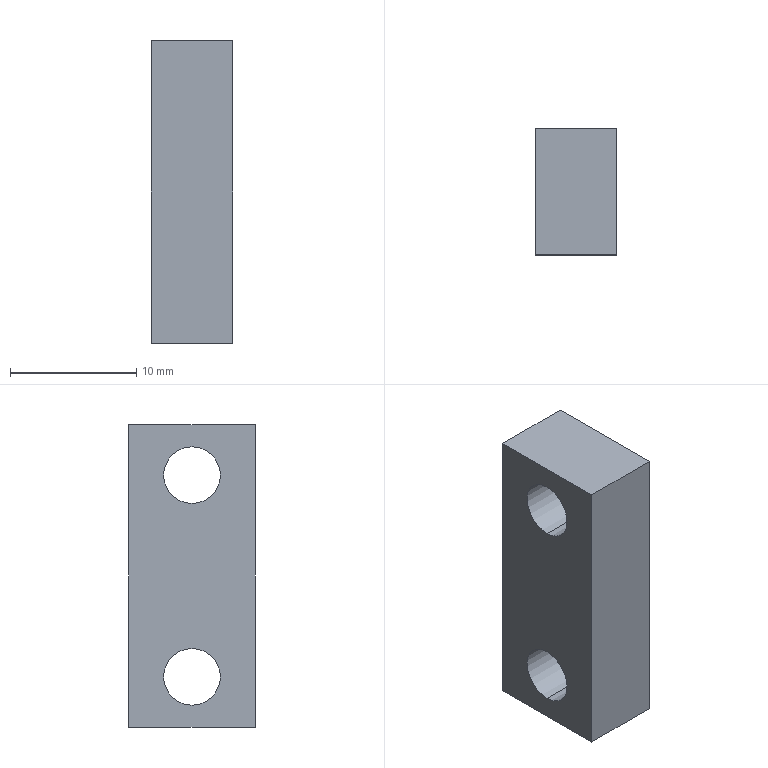Part | STEP file | PN_0044 spacer | 1 solid | 10 faces | box 6.5 x 10 x 24 mm | volume 1353 mm3 | plane 6 | cylinder 4 | commonest cylinder face diameters 4.5 x4
STEP:
#1=CARTESIAN_POINT('',(0.,0.,0.));
#2=DIRECTION('',(0.,0.,1.));
#3=DIRECTION('',(1.,0.,0.));
#4=AXIS2_PLACEMENT_3D('',#1,#2,#3);
#5=CARTESIAN_POINT('',(0.,5.,5.75));
#6=VERTEX_POINT('',#5);
#7=CARTESIAN_POINT('',(6.5,5.,5.75));
#8=VERTEX_POINT('',#7);
#9=CARTESIAN_POINT('',(6.5,5.,5.75));
#10=DIRECTION('',(1.,0.,0.));
#11=VECTOR('',#10,1.);
#12=LINE('',#9,#11);
#13=CARTESIAN_POINT('',(6.5,5.,8.));
#14=DIRECTION('',(1.,0.,0.));
#15=DIRECTION('',(0.,0.,-1.));
#16=AXIS2_PLACEMENT_3D('',#13,#14,#15);
#17=CYLINDRICAL_SURFACE('',#16,2.25);
#18=CARTESIAN_POINT('',(6.283,0.));
#19=DIRECTION('',(0.,1.));
#20=VECTOR('',#19,1.);
#21=LINE('',#18,#20);
#22=(GEOMETRIC_REPRESENTATION_CONTEXT(2)PARAMETRIC_REPRESENTATION_CONTEXT()REPRESENTATION_CONTEXT('',''));
#23=DEFINITIONAL_REPRESENTATION('',(#21),#22);
#24=PCURVE('',#17,#23);
#25=CARTESIAN_POINT('',(6.5,5.,8.));
#26=DIRECTION('',(1.,0.,0.));
#27=DIRECTION('',(0.,0.,-1.));
#28=AXIS2_PLACEMENT_3D('',#25,#26,#27);
#29=CYLINDRICAL_SURFACE('',#28,2.25);
#30=CARTESIAN_POINT('',(0.,0.));
#31=DIRECTION('',(0.,1.));
#32=VECTOR('',#31,1.);
#33=LINE('',#30,#32);
#34=(GEOMETRIC_REPRESENTATION_CONTEXT(2)PARAMETRIC_REPRESENTATION_CONTEXT()REPRESENTATION_CONTEXT('',''));
#35=DEFINITIONAL_REPRESENTATION('',(#33),#34);
#36=PCURVE('',#29,#35);
#37=SURFACE_CURVE('',#12,(#24,#36),.PCURVE_S1.);
#38=EDGE_CURVE('',#6,#8,#37,.T.);
#39=ORIENTED_EDGE('',*,*,#38,.T.);
#40=CARTESIAN_POINT('',(6.5,5.,10.25));
#41=VERTEX_POINT('',#40);
#42=CARTESIAN_POINT('',(6.5,5.,8.));
#43=DIRECTION('',(1.,0.,0.));
#44=DIRECTION('',(0.,0.,-1.));
#45=AXIS2_PLACEMENT_3D('',#42,#43,#44);
#46=CIRCLE('',#45,2.25);
#47=CARTESIAN_POINT('',(0.,0.));
#48=DIRECTION('',(1.,0.));
#49=VECTOR('',#48,1.);
#50=LINE('',#47,#49);
#51=(GEOMETRIC_REPRESENTATION_CONTEXT(2)PARAMETRIC_REPRESENTATION_CONTEXT()REPRESENTATION_CONTEXT('',''));
#52=DEFINITIONAL_REPRESENTATION('',(#50),#51);
#53=PCURVE('',#17,#52);
#54=CARTESIAN_POINT('',(6.5,0.,0.));
#55=DIRECTION('',(-1.,0.,0.));
#56=DIRECTION('',(0.,0.,1.));
#57=AXIS2_PLACEMENT_3D('',#54,#55,#56);
#58=PLANE('',#57);
#59=CARTESIAN_POINT('',(5.75,5.));
#60=CARTESIAN_POINT('',(5.75,8.897));
#61=CARTESIAN_POINT('',(9.125,6.949));
#62=CARTESIAN_POINT('',(12.5,5.));
#63=CARTESIAN_POINT('',(9.125,3.051));
#64=CARTESIAN_POINT('',(5.75,1.103));
#65=CARTESIAN_POINT('',(5.75,5.));
#66=(BOUNDED_CURVE()B_SPLINE_CURVE(2,(#59,#60,#61,#62,#63,#64,#65),.UNSPECIFIED.,.T.,.F.)B_SPLINE_CURVE_WITH_KNOTS((1,2,2,2,2,1),(-2.094,0.,2.094,4.189,6.283,8.378),.UNSPECIFIED.)CURVE()GEOMETRIC_REPRESENTATION_ITEM()RATIONAL_B_SPLINE_CURVE((1.,0.5,1.,0.5,1.,0.5,1.))REPRESENTATION_ITEM(''));
#67=(GEOMETRIC_REPRESENTATION_CONTEXT(2)PARAMETRIC_REPRESENTATION_CONTEXT()REPRESENTATION_CONTEXT('',''));
#68=DEFINITIONAL_REPRESENTATION('',(#66),#67);
#69=PCURVE('',#58,#68);
#70=SURFACE_CURVE('',#46,(#53,#69),.PCURVE_S1.);
#71=EDGE_CURVE('',#41,#8,#70,.T.);
#72=ORIENTED_EDGE('',*,*,#71,.F.);
#73=CARTESIAN_POINT('',(0.,5.,10.25));
#74=VERTEX_POINT('',#73);
#75=CARTESIAN_POINT('',(6.5,5.,10.25));
#76=DIRECTION('',(1.,0.,0.));
#77=VECTOR('',#76,1.);
#78=LINE('',#75,#77);
#79=CARTESIAN_POINT('',(3.142,0.));
#80=DIRECTION('',(0.,1.));
#81=VECTOR('',#80,1.);
#82=LINE('',#79,#81);
#83=(GEOMETRIC_REPRESENTATION_CONTEXT(2)PARAMETRIC_REPRESENTATION_CONTEXT()REPRESENTATION_CONTEXT('',''));
#84=DEFINITIONAL_REPRESENTATION('',(#82),#83);
#85=PCURVE('',#17,#84);
#86=CARTESIAN_POINT('',(3.142,0.));
#87=DIRECTION('',(0.,1.));
#88=VECTOR('',#87,1.);
#89=LINE('',#86,#88);
#90=(GEOMETRIC_REPRESENTATION_CONTEXT(2)PARAMETRIC_REPRESENTATION_CONTEXT()REPRESENTATION_CONTEXT('',''));
#91=DEFINITIONAL_REPRESENTATION('',(#89),#90);
#92=PCURVE('',#29,#91);
#93=SURFACE_CURVE('',#78,(#85,#92),.PCURVE_S1.);
#94=EDGE_CURVE('',#74,#41,#93,.T.);
#95=ORIENTED_EDGE('',*,*,#94,.F.);
#96=CARTESIAN_POINT('',(0.,5.,8.));
#97=DIRECTION('',(1.,0.,0.));
#98=DIRECTION('',(0.,0.,-1.));
#99=AXIS2_PLACEMENT_3D('',#96,#97,#98);
#100=CIRCLE('',#99,2.25);
#101=CARTESIAN_POINT('',(0.,-6.5));
#102=DIRECTION('',(1.,0.));
#103=VECTOR('',#102,1.);
#104=LINE('',#101,#103);
#105=(GEOMETRIC_REPRESENTATION_CONTEXT(2)PARAMETRIC_REPRESENTATION_CONTEXT()REPRESENTATION_CONTEXT('',''));
#106=DEFINITIONAL_REPRESENTATION('',(#104),#105);
#107=PCURVE('',#17,#106);
#108=CARTESIAN_POINT('',(0.,0.,0.));
#109=DIRECTION('',(-1.,0.,0.));
#110=DIRECTION('',(0.,0.,1.));
#111=AXIS2_PLACEMENT_3D('',#108,#109,#110);
#112=PLANE('',#111);
#113=CARTESIAN_POINT('',(5.75,5.));
#114=CARTESIAN_POINT('',(5.75,8.897));
#115=CARTESIAN_POINT('',(9.125,6.949));
#116=CARTESIAN_POINT('',(12.5,5.));
#117=CARTESIAN_POINT('',(9.125,3.051));
#118=CARTESIAN_POINT('',(5.75,1.103));
#119=CARTESIAN_POINT('',(5.75,5.));
#120=(BOUNDED_CURVE()B_SPLINE_CURVE(2,(#113,#114,#115,#116,#117,#118,#119),.UNSPECIFIED.,.T.,.F.)B_SPLINE_CURVE_WITH_KNOTS((1,2,2,2,2,1),(-2.094,0.,2.094,4.189,6.283,8.378),.UNSPECIFIED.)CURVE()GEOMETRIC_REPRESENTATION_ITEM()RATIONAL_B_SPLINE_CURVE((1.,0.5,1.,0.5,1.,0.5,1.))REPRESENTATION_ITEM(''));
#121=(GEOMETRIC_REPRESENTATION_CONTEXT(2)PARAMETRIC_REPRESENTATION_CONTEXT()REPRESENTATION_CONTEXT('',''));
#122=DEFINITIONAL_REPRESENTATION('',(#120),#121);
#123=PCURVE('',#112,#122);
#124=SURFACE_CURVE('',#100,(#107,#123),.PCURVE_S1.);
#125=EDGE_CURVE('',#74,#6,#124,.T.);
#126=ORIENTED_EDGE('',*,*,#125,.T.);
#127=EDGE_LOOP('',(#39,#72,#95,#126));
#128=FACE_BOUND('',#127,.F.);
#129=ADVANCED_FACE('',(#128),#17,.F.);
#130=CARTESIAN_POINT('',(0.,5.,-10.25));
#131=VERTEX_POINT('',#130);
#132=CARTESIAN_POINT('',(6.5,5.,-10.25));
#133=VERTEX_POINT('',#132);
#134=CARTESIAN_POINT('',(6.5,5.,-10.25));
#135=DIRECTION('',(1.,0.,0.));
#136=VECTOR('',#135,1.);
#137=LINE('',#134,#136);
#138=CARTESIAN_POINT('',(6.5,5.,-8.));
#139=DIRECTION('',(1.,0.,0.));
#140=DIRECTION('',(0.,0.,-1.));
#141=AXIS2_PLACEMENT_3D('',#138,#139,#140);
#142=CYLINDRICAL_SURFACE('',#141,2.25);
#143=CARTESIAN_POINT('',(6.283,0.));
#144=DIRECTION('',(0.,1.));
#145=VECTOR('',#144,1.);
#146=LINE('',#143,#145);
#147=(GEOMETRIC_REPRESENTATION_CONTEXT(2)PARAMETRIC_REPRESENTATION_CONTEXT()REPRESENTATION_CONTEXT('',''));
#148=DEFINITIONAL_REPRESENTATION('',(#146),#147);
#149=PCURVE('',#142,#148);
#150=CARTESIAN_POINT('',(6.5,5.,-8.));
#151=DIRECTION('',(1.,0.,0.));
#152=DIRECTION('',(0.,0.,-1.));
#153=AXIS2_PLACEMENT_3D('',#150,#151,#152);
#154=CYLINDRICAL_SURFACE('',#153,2.25);
#155=CARTESIAN_POINT('',(0.,0.));
#156=DIRECTION('',(0.,1.));
#157=VECTOR('',#156,1.);
#158=LINE('',#155,#157);
#159=(GEOMETRIC_REPRESENTATION_CONTEXT(2)PARAMETRIC_REPRESENTATION_CONTEXT()REPRESENTATION_CONTEXT('',''));
#160=DEFINITIONAL_REPRESENTATION('',(#158),#159);
#161=PCURVE('',#154,#160);
#162=SURFACE_CURVE('',#137,(#149,#161),.PCURVE_S1.);
#163=EDGE_CURVE('',#131,#133,#162,.T.);
#164=ORIENTED_EDGE('',*,*,#163,.T.);
#165=CARTESIAN_POINT('',(6.5,5.,-5.75));
#166=VERTEX_POINT('',#165);
#167=CARTESIAN_POINT('',(6.5,5.,-8.));
#168=DIRECTION('',(1.,0.,0.));
#169=DIRECTION('',(0.,0.,-1.));
#170=AXIS2_PLACEMENT_3D('',#167,#168,#169);
#171=CIRCLE('',#170,2.25);
#172=CARTESIAN_POINT('',(0.,0.));
#173=DIRECTION('',(1.,0.));
#174=VECTOR('',#173,1.);
#175=LINE('',#172,#174);
#176=(GEOMETRIC_REPRESENTATION_CONTEXT(2)PARAMETRIC_REPRESENTATION_CONTEXT()REPRESENTATION_CONTEXT('',''));
#177=DEFINITIONAL_REPRESENTATION('',(#175),#176);
#178=PCURVE('',#142,#177);
#179=CARTESIAN_POINT('',(-10.25,5.));
#180=CARTESIAN_POINT('',(-10.25,8.897));
#181=CARTESIAN_POINT('',(-6.875,6.949));
#182=CARTESIAN_POINT('',(-3.5,5.));
#183=CARTESIAN_POINT('',(-6.875,3.051));
#184=CARTESIAN_POINT('',(-10.25,1.103));
#185=CARTESIAN_POINT('',(-10.25,5.));
#186=(BOUNDED_CURVE()B_SPLINE_CURVE(2,(#179,#180,#181,#182,#183,#184,#185),.UNSPECIFIED.,.T.,.F.)B_SPLINE_CURVE_WITH_KNOTS((1,2,2,2,2,1),(-2.094,0.,2.094,4.189,6.283,8.378),.UNSPECIFIED.)CURVE()GEOMETRIC_REPRESENTATION_ITEM()RATIONAL_B_SPLINE_CURVE((1.,0.5,1.,0.5,1.,0.5,1.))REPRESENTATION_ITEM(''));
#187=(GEOMETRIC_REPRESENTATION_CONTEXT(2)PARAMETRIC_REPRESENTATION_CONTEXT()REPRESENTATION_CONTEXT('',''));
#188=DEFINITIONAL_REPRESENTATION('',(#186),#187);
#189=PCURVE('',#58,#188);
#190=SURFACE_CURVE('',#171,(#178,#189),.PCURVE_S1.);
#191=EDGE_CURVE('',#166,#133,#190,.T.);
#192=ORIENTED_EDGE('',*,*,#191,.F.);
#193=CARTESIAN_POINT('',(0.,5.,-5.75));
#194=VERTEX_POINT('',#193);
#195=CARTESIAN_POINT('',(6.5,5.,-5.75));
#196=DIRECTION('',(1.,0.,0.));
#197=VECTOR('',#196,1.);
#198=LINE('',#195,#197);
#199=CARTESIAN_POINT('',(3.142,0.));
#200=DIRECTION('',(0.,1.));
#201=VECTOR('',#200,1.);
#202=LINE('',#199,#201);
#203=(GEOMETRIC_REPRESENTATION_CONTEXT(2)PARAMETRIC_REPRESENTATION_CONTEXT()REPRESENTATION_CONTEXT('',''));
#204=DEFINITIONAL_REPRESENTATION('',(#202),#203);
#205=PCURVE('',#142,#204);
#206=CARTESIAN_POINT('',(3.142,0.));
#207=DIRECTION('',(0.,1.));
#208=VECTOR('',#207,1.);
#209=LINE('',#206,#208);
#210=(GEOMETRIC_REPRESENTATION_CONTEXT(2)PARAMETRIC_REPRESENTATION_CONTEXT()REPRESENTATION_CONTEXT('',''));
#211=DEFINITIONAL_REPRESENTATION('',(#209),#210);
#212=PCURVE('',#154,#211);
#213=SURFACE_CURVE('',#198,(#205,#212),.PCURVE_S1.);
#214=EDGE_CURVE('',#194,#166,#213,.T.);
#215=ORIENTED_EDGE('',*,*,#214,.F.);
#216=CARTESIAN_POINT('',(0.,5.,-8.));
#217=DIRECTION('',(1.,0.,0.));
#218=DIRECTION('',(0.,0.,-1.));
#219=AXIS2_PLACEMENT_3D('',#216,#217,#218);
#220=CIRCLE('',#219,2.25);
#221=CARTESIAN_POINT('',(0.,-6.5));
#222=DIRECTION('',(1.,0.));
#223=VECTOR('',#222,1.);
#224=LINE('',#221,#223);
#225=(GEOMETRIC_REPRESENTATION_CONTEXT(2)PARAMETRIC_REPRESENTATION_CONTEXT()REPRESENTATION_CONTEXT('',''));
#226=DEFINITIONAL_REPRESENTATION('',(#224),#225);
#227=PCURVE('',#142,#226);
#228=CARTESIAN_POINT('',(-10.25,5.));
#229=CARTESIAN_POINT('',(-10.25,8.897));
#230=CARTESIAN_POINT('',(-6.875,6.949));
#231=CARTESIAN_POINT('',(-3.5,5.));
#232=CARTESIAN_POINT('',(-6.875,3.051));
#233=CARTESIAN_POINT('',(-10.25,1.103));
#234=CARTESIAN_POINT('',(-10.25,5.));
#235=(BOUNDED_CURVE()B_SPLINE_CURVE(2,(#228,#229,#230,#231,#232,#233,#234),.UNSPECIFIED.,.T.,.F.)B_SPLINE_CURVE_WITH_KNOTS((1,2,2,2,2,1),(-2.094,0.,2.094,4.189,6.283,8.378),.UNSPECIFIED.)CURVE()GEOMETRIC_REPRESENTATION_ITEM()RATIONAL_B_SPLINE_CURVE((1.,0.5,1.,0.5,1.,0.5,1.))REPRESENTATION_ITEM(''));
#236=(GEOMETRIC_REPRESENTATION_CONTEXT(2)PARAMETRIC_REPRESENTATION_CONTEXT()REPRESENTATION_CONTEXT('',''));
#237=DEFINITIONAL_REPRESENTATION('',(#235),#236);
#238=PCURVE('',#112,#237);
#239=SURFACE_CURVE('',#220,(#227,#238),.PCURVE_S1.);
#240=EDGE_CURVE('',#194,#131,#239,.T.);
#241=ORIENTED_EDGE('',*,*,#240,.T.);
#242=EDGE_LOOP('',(#164,#192,#215,#241));
#243=FACE_BOUND('',#242,.F.);
#244=ADVANCED_FACE('',(#243),#142,.F.);
#245=CARTESIAN_POINT('',(0.,10.,12.));
#246=VERTEX_POINT('',#245);
#247=CARTESIAN_POINT('',(0.,0.,12.));
#248=VERTEX_POINT('',#247);
#249=CARTESIAN_POINT('',(0.,0.,12.));
#250=DIRECTION('',(0.,-1.,0.));
#251=VECTOR('',#250,1.);
#252=LINE('',#249,#251);
#253=CARTESIAN_POINT('',(6.5,0.,12.));
#254=DIRECTION('',(0.,0.,-1.));
#255=DIRECTION('',(-1.,0.,0.));
#256=AXIS2_PLACEMENT_3D('',#253,#254,#255);
#257=PLANE('',#256);
#258=CARTESIAN_POINT('',(6.5,0.));
#259=DIRECTION('',(0.,-1.));
#260=VECTOR('',#259,1.);
#261=LINE('',#258,#260);
#262=(GEOMETRIC_REPRESENTATION_CONTEXT(2)PARAMETRIC_REPRESENTATION_CONTEXT()REPRESENTATION_CONTEXT('',''));
#263=DEFINITIONAL_REPRESENTATION('',(#261),#262);
#264=PCURVE('',#257,#263);
#265=CARTESIAN_POINT('',(12.,0.));
#266=DIRECTION('',(0.,-1.));
#267=VECTOR('',#266,1.);
#268=LINE('',#265,#267);
#269=(GEOMETRIC_REPRESENTATION_CONTEXT(2)PARAMETRIC_REPRESENTATION_CONTEXT()REPRESENTATION_CONTEXT('',''));
#270=DEFINITIONAL_REPRESENTATION('',(#268),#269);
#271=PCURVE('',#112,#270);
#272=SURFACE_CURVE('',#252,(#264,#271),.PCURVE_S1.);
#273=EDGE_CURVE('',#246,#248,#272,.T.);
#274=ORIENTED_EDGE('',*,*,#273,.T.);
#275=CARTESIAN_POINT('',(6.5,0.,12.));
#276=VERTEX_POINT('',#275);
#277=CARTESIAN_POINT('',(6.5,0.,12.));
#278=DIRECTION('',(-1.,0.,0.));
#279=VECTOR('',#278,1.);
#280=LINE('',#277,#279);
#281=CARTESIAN_POINT('',(0.,0.));
#282=DIRECTION('',(1.,0.));
#283=VECTOR('',#282,1.);
#284=LINE('',#281,#283);
#285=(GEOMETRIC_REPRESENTATION_CONTEXT(2)PARAMETRIC_REPRESENTATION_CONTEXT()REPRESENTATION_CONTEXT('',''));
#286=DEFINITIONAL_REPRESENTATION('',(#284),#285);
#287=PCURVE('',#257,#286);
#288=CARTESIAN_POINT('',(6.5,0.,12.));
#289=DIRECTION('',(0.,1.,0.));
#290=DIRECTION('',(0.,0.,1.));
#291=AXIS2_PLACEMENT_3D('',#288,#289,#290);
#292=PLANE('',#291);
#293=CARTESIAN_POINT('',(0.,0.));
#294=DIRECTION('',(0.,-1.));
#295=VECTOR('',#294,1.);
#296=LINE('',#293,#295);
#297=(GEOMETRIC_REPRESENTATION_CONTEXT(2)PARAMETRIC_REPRESENTATION_CONTEXT()REPRESENTATION_CONTEXT('',''));
#298=DEFINITIONAL_REPRESENTATION('',(#296),#297);
#299=PCURVE('',#292,#298);
#300=SURFACE_CURVE('',#280,(#287,#299),.PCURVE_S1.);
#301=EDGE_CURVE('',#276,#248,#300,.T.);
#302=ORIENTED_EDGE('',*,*,#301,.F.);
#303=CARTESIAN_POINT('',(6.5,10.,12.));
#304=VERTEX_POINT('',#303);
#305=CARTESIAN_POINT('',(6.5,0.,12.));
#306=DIRECTION('',(0.,-1.,0.));
#307=VECTOR('',#306,1.);
#308=LINE('',#305,#307);
#309=CARTESIAN_POINT('',(0.,0.));
#310=DIRECTION('',(0.,-1.));
#311=VECTOR('',#310,1.);
#312=LINE('',#309,#311);
#313=(GEOMETRIC_REPRESENTATION_CONTEXT(2)PARAMETRIC_REPRESENTATION_CONTEXT()REPRESENTATION_CONTEXT('',''));
#314=DEFINITIONAL_REPRESENTATION('',(#312),#313);
#315=PCURVE('',#257,#314);
#316=CARTESIAN_POINT('',(12.,0.));
#317=DIRECTION('',(0.,-1.));
#318=VECTOR('',#317,1.);
#319=LINE('',#316,#318);
#320=(GEOMETRIC_REPRESENTATION_CONTEXT(2)PARAMETRIC_REPRESENTATION_CONTEXT()REPRESENTATION_CONTEXT('',''));
#321=DEFINITIONAL_REPRESENTATION('',(#319),#320);
#322=PCURVE('',#58,#321);
#323=SURFACE_CURVE('',#308,(#315,#322),.PCURVE_S1.);
#324=EDGE_CURVE('',#304,#276,#323,.T.);
#325=ORIENTED_EDGE('',*,*,#324,.F.);
#326=CARTESIAN_POINT('',(6.5,10.,12.));
#327=DIRECTION('',(-1.,0.,0.));
#328=VECTOR('',#327,1.);
#329=LINE('',#326,#328);
#330=CARTESIAN_POINT('',(0.,10.));
#331=DIRECTION('',(1.,0.));
#332=VECTOR('',#331,1.);
#333=LINE('',#330,#332);
#334=(GEOMETRIC_REPRESENTATION_CONTEXT(2)PARAMETRIC_REPRESENTATION_CONTEXT()REPRESENTATION_CONTEXT('',''));
#335=DEFINITIONAL_REPRESENTATION('',(#333),#334);
#336=PCURVE('',#257,#335);
#337=CARTESIAN_POINT('',(6.5,10.,12.));
#338=DIRECTION('',(0.,-1.,0.));
#339=DIRECTION('',(0.,0.,-1.));
#340=AXIS2_PLACEMENT_3D('',#337,#338,#339);
#341=PLANE('',#340);
#342=CARTESIAN_POINT('',(0.,0.));
#343=DIRECTION('',(0.,-1.));
#344=VECTOR('',#343,1.);
#345=LINE('',#342,#344);
#346=(GEOMETRIC_REPRESENTATION_CONTEXT(2)PARAMETRIC_REPRESENTATION_CONTEXT()REPRESENTATION_CONTEXT('',''));
#347=DEFINITIONAL_REPRESENTATION('',(#345),#346);
#348=PCURVE('',#341,#347);
#349=SURFACE_CURVE('',#329,(#336,#348),.PCURVE_S1.);
#350=EDGE_CURVE('',#304,#246,#349,.T.);
#351=ORIENTED_EDGE('',*,*,#350,.T.);
#352=EDGE_LOOP('',(#274,#302,#325,#351));
#353=FACE_BOUND('',#352,.T.);
#354=ADVANCED_FACE('',(#353),#257,.F.);
#355=CARTESIAN_POINT('',(0.,0.,-12.));
#356=VERTEX_POINT('',#355);
#357=CARTESIAN_POINT('',(0.,0.,12.));
#358=DIRECTION('',(0.,0.,-1.));
#359=VECTOR('',#358,1.);
#360=LINE('',#357,#359);
#361=CARTESIAN_POINT('',(0.,-6.5));
#362=DIRECTION('',(-1.,0.));
#363=VECTOR('',#362,1.);
#364=LINE('',#361,#363);
#365=(GEOMETRIC_REPRESENTATION_CONTEXT(2)PARAMETRIC_REPRESENTATION_CONTEXT()REPRESENTATION_CONTEXT('',''));
#366=DEFINITIONAL_REPRESENTATION('',(#364),#365);
#367=PCURVE('',#292,#366);
#368=CARTESIAN_POINT('',(12.,0.));
#369=DIRECTION('',(-1.,0.));
#370=VECTOR('',#369,1.);
#371=LINE('',#368,#370);
#372=(GEOMETRIC_REPRESENTATION_CONTEXT(2)PARAMETRIC_REPRESENTATION_CONTEXT()REPRESENTATION_CONTEXT('',''));
#373=DEFINITIONAL_REPRESENTATION('',(#371),#372);
#374=PCURVE('',#112,#373);
#375=SURFACE_CURVE('',#360,(#367,#374),.PCURVE_S1.);
#376=EDGE_CURVE('',#248,#356,#375,.T.);
#377=ORIENTED_EDGE('',*,*,#376,.T.);
#378=CARTESIAN_POINT('',(6.5,0.,-12.));
#379=VERTEX_POINT('',#378);
#380=CARTESIAN_POINT('',(6.5,0.,-12.));
#381=DIRECTION('',(-1.,0.,0.));
#382=VECTOR('',#381,1.);
#383=LINE('',#380,#382);
#384=CARTESIAN_POINT('',(-24.,0.));
#385=DIRECTION('',(0.,-1.));
#386=VECTOR('',#385,1.);
#387=LINE('',#384,#386);
#388=(GEOMETRIC_REPRESENTATION_CONTEXT(2)PARAMETRIC_REPRESENTATION_CONTEXT()REPRESENTATION_CONTEXT('',''));
#389=DEFINITIONAL_REPRESENTATION('',(#387),#388);
#390=PCURVE('',#292,#389);
#391=CARTESIAN_POINT('',(6.5,0.,-12.));
#392=DIRECTION('',(0.,0.,1.));
#393=DIRECTION('',(1.,0.,0.));
#394=AXIS2_PLACEMENT_3D('',#391,#392,#393);
#395=PLANE('',#394);
#396=CARTESIAN_POINT('',(0.,0.));
#397=DIRECTION('',(-1.,0.));
#398=VECTOR('',#397,1.);
#399=LINE('',#396,#398);
#400=(GEOMETRIC_REPRESENTATION_CONTEXT(2)PARAMETRIC_REPRESENTATION_CONTEXT()REPRESENTATION_CONTEXT('',''));
#401=DEFINITIONAL_REPRESENTATION('',(#399),#400);
#402=PCURVE('',#395,#401);
#403=SURFACE_CURVE('',#383,(#390,#402),.PCURVE_S1.);
#404=EDGE_CURVE('',#379,#356,#403,.T.);
#405=ORIENTED_EDGE('',*,*,#404,.F.);
#406=CARTESIAN_POINT('',(6.5,0.,12.));
#407=DIRECTION('',(0.,0.,-1.));
#408=VECTOR('',#407,1.);
#409=LINE('',#406,#408);
#410=CARTESIAN_POINT('',(0.,0.));
#411=DIRECTION('',(-1.,0.));
#412=VECTOR('',#411,1.);
#413=LINE('',#410,#412);
#414=(GEOMETRIC_REPRESENTATION_CONTEXT(2)PARAMETRIC_REPRESENTATION_CONTEXT()REPRESENTATION_CONTEXT('',''));
#415=DEFINITIONAL_REPRESENTATION('',(#413),#414);
#416=PCURVE('',#292,#415);
#417=CARTESIAN_POINT('',(12.,0.));
#418=DIRECTION('',(-1.,0.));
#419=VECTOR('',#418,1.);
#420=LINE('',#417,#419);
#421=(GEOMETRIC_REPRESENTATION_CONTEXT(2)PARAMETRIC_REPRESENTATION_CONTEXT()REPRESENTATION_CONTEXT('',''));
#422=DEFINITIONAL_REPRESENTATION('',(#420),#421);
#423=PCURVE('',#58,#422);
#424=SURFACE_CURVE('',#409,(#416,#423),.PCURVE_S1.);
#425=EDGE_CURVE('',#276,#379,#424,.T.);
#426=ORIENTED_EDGE('',*,*,#425,.F.);
#427=ORIENTED_EDGE('',*,*,#301,.T.);
#428=EDGE_LOOP('',(#377,#405,#426,#427));
#429=FACE_BOUND('',#428,.T.);
#430=ADVANCED_FACE('',(#429),#292,.F.);
#431=CARTESIAN_POINT('',(0.,10.,-12.));
#432=VERTEX_POINT('',#431);
#433=CARTESIAN_POINT('',(0.,0.,-12.));
#434=DIRECTION('',(0.,1.,0.));
#435=VECTOR('',#434,1.);
#436=LINE('',#433,#435);
#437=CARTESIAN_POINT('',(-6.5,0.));
#438=DIRECTION('',(0.,1.));
#439=VECTOR('',#438,1.);
#440=LINE('',#437,#439);
#441=(GEOMETRIC_REPRESENTATION_CONTEXT(2)PARAMETRIC_REPRESENTATION_CONTEXT()REPRESENTATION_CONTEXT('',''));
#442=DEFINITIONAL_REPRESENTATION('',(#440),#441);
#443=PCURVE('',#395,#442);
#444=CARTESIAN_POINT('',(-12.,0.));
#445=DIRECTION('',(0.,1.));
#446=VECTOR('',#445,1.);
#447=LINE('',#444,#446);
#448=(GEOMETRIC_REPRESENTATION_CONTEXT(2)PARAMETRIC_REPRESENTATION_CONTEXT()REPRESENTATION_CONTEXT('',''));
#449=DEFINITIONAL_REPRESENTATION('',(#447),#448);
#450=PCURVE('',#112,#449);
#451=SURFACE_CURVE('',#436,(#443,#450),.PCURVE_S1.);
#452=EDGE_CURVE('',#356,#432,#451,.T.);
#453=ORIENTED_EDGE('',*,*,#452,.T.);
#454=CARTESIAN_POINT('',(6.5,10.,-12.));
#455=VERTEX_POINT('',#454);
#456=CARTESIAN_POINT('',(6.5,10.,-12.));
#457=DIRECTION('',(-1.,0.,0.));
#458=VECTOR('',#457,1.);
#459=LINE('',#456,#458);
#460=CARTESIAN_POINT('',(0.,10.));
#461=DIRECTION('',(-1.,0.));
#462=VECTOR('',#461,1.);
#463=LINE('',#460,#462);
#464=(GEOMETRIC_REPRESENTATION_CONTEXT(2)PARAMETRIC_REPRESENTATION_CONTEXT()REPRESENTATION_CONTEXT('',''));
#465=DEFINITIONAL_REPRESENTATION('',(#463),#464);
#466=PCURVE('',#395,#465);
#467=CARTESIAN_POINT('',(24.,0.));
#468=DIRECTION('',(0.,-1.));
#469=VECTOR('',#468,1.);
#470=LINE('',#467,#469);
#471=(GEOMETRIC_REPRESENTATION_CONTEXT(2)PARAMETRIC_REPRESENTATION_CONTEXT()REPRESENTATION_CONTEXT('',''));
#472=DEFINITIONAL_REPRESENTATION('',(#470),#471);
#473=PCURVE('',#341,#472);
#474=SURFACE_CURVE('',#459,(#466,#473),.PCURVE_S1.);
#475=EDGE_CURVE('',#455,#432,#474,.T.);
#476=ORIENTED_EDGE('',*,*,#475,.F.);
#477=CARTESIAN_POINT('',(6.5,0.,-12.));
#478=DIRECTION('',(0.,1.,0.));
#479=VECTOR('',#478,1.);
#480=LINE('',#477,#479);
#481=CARTESIAN_POINT('',(0.,0.));
#482=DIRECTION('',(0.,1.));
#483=VECTOR('',#482,1.);
#484=LINE('',#481,#483);
#485=(GEOMETRIC_REPRESENTATION_CONTEXT(2)PARAMETRIC_REPRESENTATION_CONTEXT()REPRESENTATION_CONTEXT('',''));
#486=DEFINITIONAL_REPRESENTATION('',(#484),#485);
#487=PCURVE('',#395,#486);
#488=CARTESIAN_POINT('',(-12.,0.));
#489=DIRECTION('',(0.,1.));
#490=VECTOR('',#489,1.);
#491=LINE('',#488,#490);
#492=(GEOMETRIC_REPRESENTATION_CONTEXT(2)PARAMETRIC_REPRESENTATION_CONTEXT()REPRESENTATION_CONTEXT('',''));
#493=DEFINITIONAL_REPRESENTATION('',(#491),#492);
#494=PCURVE('',#58,#493);
#495=SURFACE_CURVE('',#480,(#487,#494),.PCURVE_S1.);
#496=EDGE_CURVE('',#379,#455,#495,.T.);
#497=ORIENTED_EDGE('',*,*,#496,.F.);
#498=ORIENTED_EDGE('',*,*,#404,.T.);
#499=EDGE_LOOP('',(#453,#476,#497,#498));
#500=FACE_BOUND('',#499,.T.);
#501=ADVANCED_FACE('',(#500),#395,.F.);
#502=CARTESIAN_POINT('',(0.,10.,12.));
#503=DIRECTION('',(0.,0.,1.));
#504=VECTOR('',#503,1.);
#505=LINE('',#502,#504);
#506=CARTESIAN_POINT('',(0.,-6.5));
#507=DIRECTION('',(-1.,0.));
#508=VECTOR('',#507,1.);
#509=LINE('',#506,#508);
#510=(GEOMETRIC_REPRESENTATION_CONTEXT(2)PARAMETRIC_REPRESENTATION_CONTEXT()REPRESENTATION_CONTEXT('',''));
#511=DEFINITIONAL_REPRESENTATION('',(#509),#510);
#512=PCURVE('',#341,#511);
#513=CARTESIAN_POINT('',(12.,10.));
#514=DIRECTION('',(1.,0.));
#515=VECTOR('',#514,1.);
#516=LINE('',#513,#515);
#517=(GEOMETRIC_REPRESENTATION_CONTEXT(2)PARAMETRIC_REPRESENTATION_CONTEXT()REPRESENTATION_CONTEXT('',''));
#518=DEFINITIONAL_REPRESENTATION('',(#516),#517);
#519=PCURVE('',#112,#518);
#520=SURFACE_CURVE('',#505,(#512,#519),.PCURVE_S1.);
#521=EDGE_CURVE('',#432,#246,#520,.T.);
#522=ORIENTED_EDGE('',*,*,#521,.T.);
#523=ORIENTED_EDGE('',*,*,#350,.F.);
#524=CARTESIAN_POINT('',(6.5,10.,12.));
#525=DIRECTION('',(0.,0.,1.));
#526=VECTOR('',#525,1.);
#527=LINE('',#524,#526);
#528=CARTESIAN_POINT('',(0.,0.));
#529=DIRECTION('',(-1.,0.));
#530=VECTOR('',#529,1.);
#531=LINE('',#528,#530);
#532=(GEOMETRIC_REPRESENTATION_CONTEXT(2)PARAMETRIC_REPRESENTATION_CONTEXT()REPRESENTATION_CONTEXT('',''));
#533=DEFINITIONAL_REPRESENTATION('',(#531),#532);
#534=PCURVE('',#341,#533);
#535=CARTESIAN_POINT('',(12.,10.));
#536=DIRECTION('',(1.,0.));
#537=VECTOR('',#536,1.);
#538=LINE('',#535,#537);
#539=(GEOMETRIC_REPRESENTATION_CONTEXT(2)PARAMETRIC_REPRESENTATION_CONTEXT()REPRESENTATION_CONTEXT('',''));
#540=DEFINITIONAL_REPRESENTATION('',(#538),#539);
#541=PCURVE('',#58,#540);
#542=SURFACE_CURVE('',#527,(#534,#541),.PCURVE_S1.);
#543=EDGE_CURVE('',#455,#304,#542,.T.);
#544=ORIENTED_EDGE('',*,*,#543,.F.);
#545=ORIENTED_EDGE('',*,*,#475,.T.);
#546=EDGE_LOOP('',(#522,#523,#544,#545));
#547=FACE_BOUND('',#546,.T.);
#548=ADVANCED_FACE('',(#547),#341,.F.);
#549=CARTESIAN_POINT('',(6.5,5.,8.));
#550=DIRECTION('',(1.,0.,0.));
#551=DIRECTION('',(0.,0.,-1.));
#552=AXIS2_PLACEMENT_3D('',#549,#550,#551);
#553=CIRCLE('',#552,2.25);
#554=CARTESIAN_POINT('',(5.75,5.));
#555=CARTESIAN_POINT('',(5.75,8.897));
#556=CARTESIAN_POINT('',(9.125,6.949));
#557=CARTESIAN_POINT('',(12.5,5.));
#558=CARTESIAN_POINT('',(9.125,3.051));
#559=CARTESIAN_POINT('',(5.75,1.103));
#560=CARTESIAN_POINT('',(5.75,5.));
#561=(BOUNDED_CURVE()B_SPLINE_CURVE(2,(#554,#555,#556,#557,#558,#559,#560),.UNSPECIFIED.,.T.,.F.)B_SPLINE_CURVE_WITH_KNOTS((1,2,2,2,2,1),(-2.094,0.,2.094,4.189,6.283,8.378),.UNSPECIFIED.)CURVE()GEOMETRIC_REPRESENTATION_ITEM()RATIONAL_B_SPLINE_CURVE((1.,0.5,1.,0.5,1.,0.5,1.))REPRESENTATION_ITEM(''));
#562=(GEOMETRIC_REPRESENTATION_CONTEXT(2)PARAMETRIC_REPRESENTATION_CONTEXT()REPRESENTATION_CONTEXT('',''));
#563=DEFINITIONAL_REPRESENTATION('',(#561),#562);
#564=PCURVE('',#58,#563);
#565=CARTESIAN_POINT('',(0.,0.));
#566=DIRECTION('',(1.,0.));
#567=VECTOR('',#566,1.);
#568=LINE('',#565,#567);
#569=(GEOMETRIC_REPRESENTATION_CONTEXT(2)PARAMETRIC_REPRESENTATION_CONTEXT()REPRESENTATION_CONTEXT('',''));
#570=DEFINITIONAL_REPRESENTATION('',(#568),#569);
#571=PCURVE('',#29,#570);
#572=SURFACE_CURVE('',#553,(#564,#571),.PCURVE_S1.);
#573=EDGE_CURVE('',#8,#41,#572,.T.);
#574=ORIENTED_EDGE('',*,*,#573,.F.);
#575=ORIENTED_EDGE('',*,*,#71,.F.);
#576=EDGE_LOOP('',(#574,#575));
#577=FACE_BOUND('',#576,.T.);
#578=CARTESIAN_POINT('',(6.5,5.,-8.));
#579=DIRECTION('',(1.,0.,0.));
#580=DIRECTION('',(0.,0.,-1.));
#581=AXIS2_PLACEMENT_3D('',#578,#579,#580);
#582=CIRCLE('',#581,2.25);
#583=CARTESIAN_POINT('',(-10.25,5.));
#584=CARTESIAN_POINT('',(-10.25,8.897));
#585=CARTESIAN_POINT('',(-6.875,6.949));
#586=CARTESIAN_POINT('',(-3.5,5.));
#587=CARTESIAN_POINT('',(-6.875,3.051));
#588=CARTESIAN_POINT('',(-10.25,1.103));
#589=CARTESIAN_POINT('',(-10.25,5.));
#590=(BOUNDED_CURVE()B_SPLINE_CURVE(2,(#583,#584,#585,#586,#587,#588,#589),.UNSPECIFIED.,.T.,.F.)B_SPLINE_CURVE_WITH_KNOTS((1,2,2,2,2,1),(-2.094,0.,2.094,4.189,6.283,8.378),.UNSPECIFIED.)CURVE()GEOMETRIC_REPRESENTATION_ITEM()RATIONAL_B_SPLINE_CURVE((1.,0.5,1.,0.5,1.,0.5,1.))REPRESENTATION_ITEM(''));
#591=(GEOMETRIC_REPRESENTATION_CONTEXT(2)PARAMETRIC_REPRESENTATION_CONTEXT()REPRESENTATION_CONTEXT('',''));
#592=DEFINITIONAL_REPRESENTATION('',(#590),#591);
#593=PCURVE('',#58,#592);
#594=CARTESIAN_POINT('',(0.,0.));
#595=DIRECTION('',(1.,0.));
#596=VECTOR('',#595,1.);
#597=LINE('',#594,#596);
#598=(GEOMETRIC_REPRESENTATION_CONTEXT(2)PARAMETRIC_REPRESENTATION_CONTEXT()REPRESENTATION_CONTEXT('',''));
#599=DEFINITIONAL_REPRESENTATION('',(#597),#598);
#600=PCURVE('',#154,#599);
#601=SURFACE_CURVE('',#582,(#593,#600),.PCURVE_S1.);
#602=EDGE_CURVE('',#133,#166,#601,.T.);
#603=ORIENTED_EDGE('',*,*,#602,.F.);
#604=ORIENTED_EDGE('',*,*,#191,.F.);
#605=EDGE_LOOP('',(#603,#604));
#606=FACE_BOUND('',#605,.T.);
#607=ORIENTED_EDGE('',*,*,#324,.T.);
#608=ORIENTED_EDGE('',*,*,#425,.T.);
#609=ORIENTED_EDGE('',*,*,#496,.T.);
#610=ORIENTED_EDGE('',*,*,#543,.T.);
#611=EDGE_LOOP('',(#607,#608,#609,#610));
#612=FACE_BOUND('',#611,.T.);
#613=ADVANCED_FACE('',(#577,#606,#612),#58,.F.);
#614=CARTESIAN_POINT('',(0.,5.,8.));
#615=DIRECTION('',(1.,0.,0.));
#616=DIRECTION('',(0.,0.,-1.));
#617=AXIS2_PLACEMENT_3D('',#614,#615,#616);
#618=CIRCLE('',#617,2.25);
#619=CARTESIAN_POINT('',(5.75,5.));
#620=CARTESIAN_POINT('',(5.75,8.897));
#621=CARTESIAN_POINT('',(9.125,6.949));
#622=CARTESIAN_POINT('',(12.5,5.));
#623=CARTESIAN_POINT('',(9.125,3.051));
#624=CARTESIAN_POINT('',(5.75,1.103));
#625=CARTESIAN_POINT('',(5.75,5.));
#626=(BOUNDED_CURVE()B_SPLINE_CURVE(2,(#619,#620,#621,#622,#623,#624,#625),.UNSPECIFIED.,.T.,.F.)B_SPLINE_CURVE_WITH_KNOTS((1,2,2,2,2,1),(-2.094,0.,2.094,4.189,6.283,8.378),.UNSPECIFIED.)CURVE()GEOMETRIC_REPRESENTATION_ITEM()RATIONAL_B_SPLINE_CURVE((1.,0.5,1.,0.5,1.,0.5,1.))REPRESENTATION_ITEM(''));
#627=(GEOMETRIC_REPRESENTATION_CONTEXT(2)PARAMETRIC_REPRESENTATION_CONTEXT()REPRESENTATION_CONTEXT('',''));
#628=DEFINITIONAL_REPRESENTATION('',(#626),#627);
#629=PCURVE('',#112,#628);
#630=CARTESIAN_POINT('',(0.,-6.5));
#631=DIRECTION('',(1.,0.));
#632=VECTOR('',#631,1.);
#633=LINE('',#630,#632);
#634=(GEOMETRIC_REPRESENTATION_CONTEXT(2)PARAMETRIC_REPRESENTATION_CONTEXT()REPRESENTATION_CONTEXT('',''));
#635=DEFINITIONAL_REPRESENTATION('',(#633),#634);
#636=PCURVE('',#29,#635);
#637=SURFACE_CURVE('',#618,(#629,#636),.PCURVE_S1.);
#638=EDGE_CURVE('',#6,#74,#637,.T.);
#639=ORIENTED_EDGE('',*,*,#638,.T.);
#640=ORIENTED_EDGE('',*,*,#125,.T.);
#641=EDGE_LOOP('',(#639,#640));
#642=FACE_BOUND('',#641,.T.);
#643=CARTESIAN_POINT('',(0.,5.,-8.));
#644=DIRECTION('',(1.,0.,0.));
#645=DIRECTION('',(0.,0.,-1.));
#646=AXIS2_PLACEMENT_3D('',#643,#644,#645);
#647=CIRCLE('',#646,2.25);
#648=CARTESIAN_POINT('',(-10.25,5.));
#649=CARTESIAN_POINT('',(-10.25,8.897));
#650=CARTESIAN_POINT('',(-6.875,6.949));
#651=CARTESIAN_POINT('',(-3.5,5.));
#652=CARTESIAN_POINT('',(-6.875,3.051));
#653=CARTESIAN_POINT('',(-10.25,1.103));
#654=CARTESIAN_POINT('',(-10.25,5.));
#655=(BOUNDED_CURVE()B_SPLINE_CURVE(2,(#648,#649,#650,#651,#652,#653,#654),.UNSPECIFIED.,.T.,.F.)B_SPLINE_CURVE_WITH_KNOTS((1,2,2,2,2,1),(-2.094,0.,2.094,4.189,6.283,8.378),.UNSPECIFIED.)CURVE()GEOMETRIC_REPRESENTATION_ITEM()RATIONAL_B_SPLINE_CURVE((1.,0.5,1.,0.5,1.,0.5,1.))REPRESENTATION_ITEM(''));
#656=(GEOMETRIC_REPRESENTATION_CONTEXT(2)PARAMETRIC_REPRESENTATION_CONTEXT()REPRESENTATION_CONTEXT('',''));
#657=DEFINITIONAL_REPRESENTATION('',(#655),#656);
#658=PCURVE('',#112,#657);
#659=CARTESIAN_POINT('',(0.,-6.5));
#660=DIRECTION('',(1.,0.));
#661=VECTOR('',#660,1.);
#662=LINE('',#659,#661);
#663=(GEOMETRIC_REPRESENTATION_CONTEXT(2)PARAMETRIC_REPRESENTATION_CONTEXT()REPRESENTATION_CONTEXT('',''));
#664=DEFINITIONAL_REPRESENTATION('',(#662),#663);
#665=PCURVE('',#154,#664);
#666=SURFACE_CURVE('',#647,(#658,#665),.PCURVE_S1.);
#667=EDGE_CURVE('',#131,#194,#666,.T.);
#668=ORIENTED_EDGE('',*,*,#667,.T.);
#669=ORIENTED_EDGE('',*,*,#240,.T.);
#670=EDGE_LOOP('',(#668,#669));
#671=FACE_BOUND('',#670,.T.);
#672=ORIENTED_EDGE('',*,*,#273,.F.);
#673=ORIENTED_EDGE('',*,*,#521,.F.);
#674=ORIENTED_EDGE('',*,*,#452,.F.);
#675=ORIENTED_EDGE('',*,*,#376,.F.);
#676=EDGE_LOOP('',(#672,#673,#674,#675));
#677=FACE_BOUND('',#676,.T.);
#678=ADVANCED_FACE('',(#642,#671,#677),#112,.T.);
#679=ORIENTED_EDGE('',*,*,#602,.F.);
#680=ORIENTED_EDGE('',*,*,#163,.F.);
#681=ORIENTED_EDGE('',*,*,#667,.T.);
#682=ORIENTED_EDGE('',*,*,#214,.T.);
#683=EDGE_LOOP('',(#679,#680,#681,#682));
#684=FACE_BOUND('',#683,.F.);
#685=ADVANCED_FACE('',(#684),#154,.F.);
#686=ORIENTED_EDGE('',*,*,#573,.F.);
#687=ORIENTED_EDGE('',*,*,#38,.F.);
#688=ORIENTED_EDGE('',*,*,#638,.T.);
#689=ORIENTED_EDGE('',*,*,#94,.T.);
#690=EDGE_LOOP('',(#686,#687,#688,#689));
#691=FACE_BOUND('',#690,.F.);
#692=ADVANCED_FACE('',(#691),#29,.F.);
#693=CLOSED_SHELL('',(#129,#244,#354,#430,#501,#548,#613,#678,#685,#692));
#694=MANIFOLD_SOLID_BREP('',#693);
#695=(LENGTH_UNIT()NAMED_UNIT(*)SI_UNIT(.MILLI.,.METRE.));
#696=UNCERTAINTY_MEASURE_WITH_UNIT(LENGTH_MEASURE(0.0000001),#695,'','');
#697=(NAMED_UNIT(*)PLANE_ANGLE_UNIT()SI_UNIT($,.RADIAN.));
#698=(NAMED_UNIT(*)SI_UNIT($,.STERADIAN.)SOLID_ANGLE_UNIT());
#699=(GEOMETRIC_REPRESENTATION_CONTEXT(3)GLOBAL_UNCERTAINTY_ASSIGNED_CONTEXT((#696))GLOBAL_UNIT_ASSIGNED_CONTEXT((#695,#697,#698))REPRESENTATION_CONTEXT('',''));
#700=ADVANCED_BREP_SHAPE_REPRESENTATION('',(#4,#694),#699);